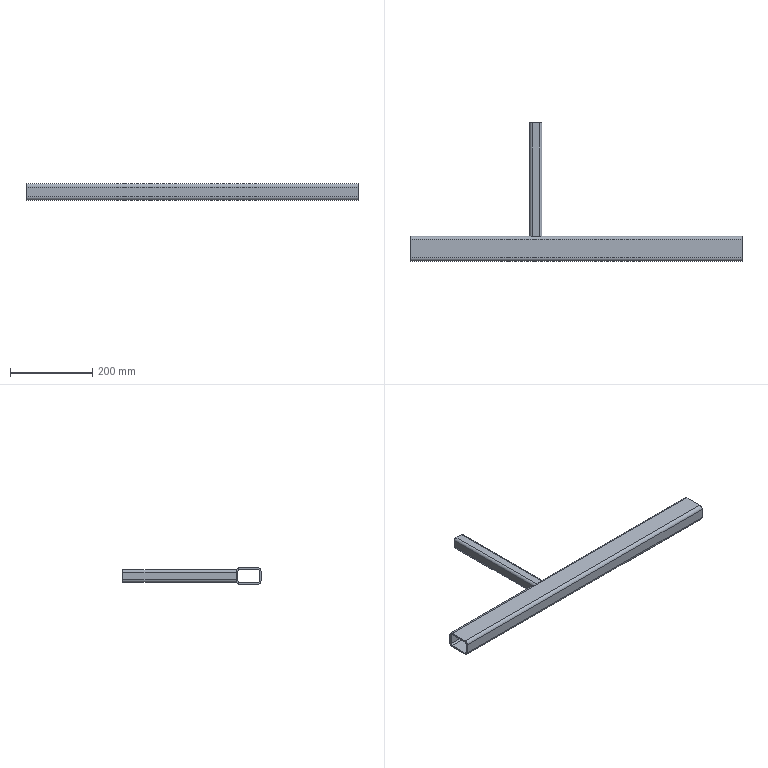Part | SolidWorks | features WeldMemberFeat 2, WeldCornerFeat 1, WeldmentFeature 1 | 2 solids | 36 faces | box 805 x 335 x 40 mm | volume 647000 mm3 | plane 20 | cylinder 16 | commonest cylinder face diameters 5.6 x4 8 x4 12 x4 16 x4
STEP:
#1=CARTESIAN_POINT('',(0.,-22.,20.));
#2=VERTEX_POINT('',#1);
#3=CARTESIAN_POINT('',(0.,-30.,12.));
#4=VERTEX_POINT('',#3);
#5=CARTESIAN_POINT('',(0.,-22.,12.));
#6=DIRECTION('',(1.,0.,0.));
#7=DIRECTION('',(0.,0.,-1.));
#8=AXIS2_PLACEMENT_3D('',#5,#6,#7);
#9=CIRCLE('',#8,8.);
#10=EDGE_CURVE('',#2,#4,#9,.T.);
#11=ORIENTED_EDGE('',*,*,#10,.T.);
#12=CARTESIAN_POINT('',(805.,-30.,12.));
#13=VERTEX_POINT('',#12);
#14=CARTESIAN_POINT('',(805.,-30.,12.));
#15=DIRECTION('',(-1.,0.,0.));
#16=VECTOR('',#15,1000.);
#17=LINE('',#14,#16);
#18=EDGE_CURVE('',#13,#4,#17,.T.);
#19=ORIENTED_EDGE('',*,*,#18,.F.);
#20=CARTESIAN_POINT('',(805.,-22.,20.));
#21=VERTEX_POINT('',#20);
#22=CARTESIAN_POINT('',(805.,-22.,12.));
#23=DIRECTION('',(1.,0.,0.));
#24=DIRECTION('',(0.,0.,-1.));
#25=AXIS2_PLACEMENT_3D('',#22,#23,#24);
#26=CIRCLE('',#25,8.);
#27=EDGE_CURVE('',#21,#13,#26,.T.);
#28=ORIENTED_EDGE('',*,*,#27,.F.);
#29=CARTESIAN_POINT('',(805.,-22.,20.));
#30=DIRECTION('',(-1.,0.,0.));
#31=VECTOR('',#30,1000.);
#32=LINE('',#29,#31);
#33=EDGE_CURVE('',#21,#2,#32,.T.);
#34=ORIENTED_EDGE('',*,*,#33,.T.);
#35=EDGE_LOOP('',(#11,#19,#28,#34));
#36=FACE_OUTER_BOUND('',#35,.T.);
#37=CARTESIAN_POINT('',(805.,-22.,12.));
#38=DIRECTION('',(-1.,0.,0.));
#39=DIRECTION('',(0.,0.,1.));
#40=AXIS2_PLACEMENT_3D('',#37,#38,#39);
#41=CYLINDRICAL_SURFACE('',#40,8.);
#42=ADVANCED_FACE('',(#36),#41,.T.);
#43=CARTESIAN_POINT('',(0.,-30.,-12.));
#44=VERTEX_POINT('',#43);
#45=CARTESIAN_POINT('',(0.,-30.,12.));
#46=DIRECTION('',(0.,0.,-1.));
#47=VECTOR('',#46,1000.);
#48=LINE('',#45,#47);
#49=EDGE_CURVE('',#4,#44,#48,.T.);
#50=ORIENTED_EDGE('',*,*,#49,.T.);
#51=CARTESIAN_POINT('',(805.,-30.,-12.));
#52=VERTEX_POINT('',#51);
#53=CARTESIAN_POINT('',(805.,-30.,-12.));
#54=DIRECTION('',(-1.,0.,0.));
#55=VECTOR('',#54,1000.);
#56=LINE('',#53,#55);
#57=EDGE_CURVE('',#52,#44,#56,.T.);
#58=ORIENTED_EDGE('',*,*,#57,.F.);
#59=CARTESIAN_POINT('',(805.,-30.,12.));
#60=DIRECTION('',(0.,0.,-1.));
#61=VECTOR('',#60,1000.);
#62=LINE('',#59,#61);
#63=EDGE_CURVE('',#13,#52,#62,.T.);
#64=ORIENTED_EDGE('',*,*,#63,.F.);
#65=ORIENTED_EDGE('',*,*,#18,.T.);
#66=EDGE_LOOP('',(#50,#58,#64,#65));
#67=FACE_OUTER_BOUND('',#66,.T.);
#68=CARTESIAN_POINT('',(805.,-30.,12.));
#69=DIRECTION('',(0.,1.,0.));
#70=DIRECTION('',(0.,0.,1.));
#71=AXIS2_PLACEMENT_3D('',#68,#69,#70);
#72=PLANE('',#71);
#73=ADVANCED_FACE('',(#67),#72,.F.);
#74=CARTESIAN_POINT('',(0.,-22.,-20.));
#75=VERTEX_POINT('',#74);
#76=CARTESIAN_POINT('',(0.,-22.,-12.));
#77=DIRECTION('',(1.,0.,0.));
#78=DIRECTION('',(0.,0.,-1.));
#79=AXIS2_PLACEMENT_3D('',#76,#77,#78);
#80=CIRCLE('',#79,8.);
#81=EDGE_CURVE('',#44,#75,#80,.T.);
#82=ORIENTED_EDGE('',*,*,#81,.T.);
#83=CARTESIAN_POINT('',(805.,-22.,-20.));
#84=VERTEX_POINT('',#83);
#85=CARTESIAN_POINT('',(805.,-22.,-20.));
#86=DIRECTION('',(-1.,0.,0.));
#87=VECTOR('',#86,1000.);
#88=LINE('',#85,#87);
#89=EDGE_CURVE('',#84,#75,#88,.T.);
#90=ORIENTED_EDGE('',*,*,#89,.F.);
#91=CARTESIAN_POINT('',(805.,-22.,-12.));
#92=DIRECTION('',(1.,0.,0.));
#93=DIRECTION('',(0.,0.,-1.));
#94=AXIS2_PLACEMENT_3D('',#91,#92,#93);
#95=CIRCLE('',#94,8.);
#96=EDGE_CURVE('',#52,#84,#95,.T.);
#97=ORIENTED_EDGE('',*,*,#96,.F.);
#98=ORIENTED_EDGE('',*,*,#57,.T.);
#99=EDGE_LOOP('',(#82,#90,#97,#98));
#100=FACE_OUTER_BOUND('',#99,.T.);
#101=CARTESIAN_POINT('',(805.,-22.,-12.));
#102=DIRECTION('',(-1.,0.,0.));
#103=DIRECTION('',(0.,0.,1.));
#104=AXIS2_PLACEMENT_3D('',#101,#102,#103);
#105=CYLINDRICAL_SURFACE('',#104,8.);
#106=ADVANCED_FACE('',(#100),#105,.T.);
#107=CARTESIAN_POINT('',(0.,22.,-20.));
#108=VERTEX_POINT('',#107);
#109=CARTESIAN_POINT('',(0.,22.,-20.));
#110=DIRECTION('',(0.,1.,0.));
#111=VECTOR('',#110,1000.);
#112=LINE('',#109,#111);
#113=EDGE_CURVE('',#75,#108,#112,.T.);
#114=ORIENTED_EDGE('',*,*,#113,.T.);
#115=CARTESIAN_POINT('',(805.,22.,-20.));
#116=VERTEX_POINT('',#115);
#117=CARTESIAN_POINT('',(805.,22.,-20.));
#118=DIRECTION('',(-1.,0.,0.));
#119=VECTOR('',#118,1000.);
#120=LINE('',#117,#119);
#121=EDGE_CURVE('',#116,#108,#120,.T.);
#122=ORIENTED_EDGE('',*,*,#121,.F.);
#123=CARTESIAN_POINT('',(805.,22.,-20.));
#124=DIRECTION('',(0.,1.,0.));
#125=VECTOR('',#124,1000.);
#126=LINE('',#123,#125);
#127=EDGE_CURVE('',#84,#116,#126,.T.);
#128=ORIENTED_EDGE('',*,*,#127,.F.);
#129=ORIENTED_EDGE('',*,*,#89,.T.);
#130=EDGE_LOOP('',(#114,#122,#128,#129));
#131=FACE_OUTER_BOUND('',#130,.T.);
#132=CARTESIAN_POINT('',(805.,22.,-20.));
#133=DIRECTION('',(0.,0.,1.));
#134=DIRECTION('',(0.,-1.,0.));
#135=AXIS2_PLACEMENT_3D('',#132,#133,#134);
#136=PLANE('',#135);
#137=ADVANCED_FACE('',(#131),#136,.F.);
#138=CARTESIAN_POINT('',(0.,30.,-12.));
#139=VERTEX_POINT('',#138);
#140=CARTESIAN_POINT('',(0.,22.,-12.));
#141=DIRECTION('',(1.,0.,0.));
#142=DIRECTION('',(0.,0.,-1.));
#143=AXIS2_PLACEMENT_3D('',#140,#141,#142);
#144=CIRCLE('',#143,8.);
#145=EDGE_CURVE('',#108,#139,#144,.T.);
#146=ORIENTED_EDGE('',*,*,#145,.T.);
#147=CARTESIAN_POINT('',(805.,30.,-12.));
#148=VERTEX_POINT('',#147);
#149=CARTESIAN_POINT('',(805.,30.,-12.));
#150=DIRECTION('',(-1.,0.,0.));
#151=VECTOR('',#150,1000.);
#152=LINE('',#149,#151);
#153=EDGE_CURVE('',#148,#139,#152,.T.);
#154=ORIENTED_EDGE('',*,*,#153,.F.);
#155=CARTESIAN_POINT('',(805.,22.,-12.));
#156=DIRECTION('',(1.,0.,0.));
#157=DIRECTION('',(0.,0.,-1.));
#158=AXIS2_PLACEMENT_3D('',#155,#156,#157);
#159=CIRCLE('',#158,8.);
#160=EDGE_CURVE('',#116,#148,#159,.T.);
#161=ORIENTED_EDGE('',*,*,#160,.F.);
#162=ORIENTED_EDGE('',*,*,#121,.T.);
#163=EDGE_LOOP('',(#146,#154,#161,#162));
#164=FACE_OUTER_BOUND('',#163,.T.);
#165=CARTESIAN_POINT('',(805.,22.,-12.));
#166=DIRECTION('',(-1.,0.,0.));
#167=DIRECTION('',(0.,0.,1.));
#168=AXIS2_PLACEMENT_3D('',#165,#166,#167);
#169=CYLINDRICAL_SURFACE('',#168,8.);
#170=ADVANCED_FACE('',(#164),#169,.T.);
#171=CARTESIAN_POINT('',(0.,30.,12.));
#172=VERTEX_POINT('',#171);
#173=CARTESIAN_POINT('',(0.,30.,-12.));
#174=DIRECTION('',(0.,0.,1.));
#175=VECTOR('',#174,1000.);
#176=LINE('',#173,#175);
#177=EDGE_CURVE('',#139,#172,#176,.T.);
#178=ORIENTED_EDGE('',*,*,#177,.T.);
#179=CARTESIAN_POINT('',(805.,30.,12.));
#180=VERTEX_POINT('',#179);
#181=CARTESIAN_POINT('',(805.,30.,12.));
#182=DIRECTION('',(-1.,0.,0.));
#183=VECTOR('',#182,1000.);
#184=LINE('',#181,#183);
#185=EDGE_CURVE('',#180,#172,#184,.T.);
#186=ORIENTED_EDGE('',*,*,#185,.F.);
#187=CARTESIAN_POINT('',(805.,30.,-12.));
#188=DIRECTION('',(0.,0.,1.));
#189=VECTOR('',#188,1000.);
#190=LINE('',#187,#189);
#191=EDGE_CURVE('',#148,#180,#190,.T.);
#192=ORIENTED_EDGE('',*,*,#191,.F.);
#193=ORIENTED_EDGE('',*,*,#153,.T.);
#194=EDGE_LOOP('',(#178,#186,#192,#193));
#195=FACE_OUTER_BOUND('',#194,.T.);
#196=CARTESIAN_POINT('',(805.,30.,-12.));
#197=DIRECTION('',(0.,-1.,0.));
#198=DIRECTION('',(0.,0.,-1.));
#199=AXIS2_PLACEMENT_3D('',#196,#197,#198);
#200=PLANE('',#199);
#201=ADVANCED_FACE('',(#195),#200,.F.);
#202=CARTESIAN_POINT('',(0.,22.,20.));
#203=VERTEX_POINT('',#202);
#204=CARTESIAN_POINT('',(0.,22.,12.));
#205=DIRECTION('',(1.,0.,0.));
#206=DIRECTION('',(0.,0.,-1.));
#207=AXIS2_PLACEMENT_3D('',#204,#205,#206);
#208=CIRCLE('',#207,8.);
#209=EDGE_CURVE('',#172,#203,#208,.T.);
#210=ORIENTED_EDGE('',*,*,#209,.T.);
#211=CARTESIAN_POINT('',(805.,22.,20.));
#212=VERTEX_POINT('',#211);
#213=CARTESIAN_POINT('',(805.,22.,20.));
#214=DIRECTION('',(-1.,0.,0.));
#215=VECTOR('',#214,1000.);
#216=LINE('',#213,#215);
#217=EDGE_CURVE('',#212,#203,#216,.T.);
#218=ORIENTED_EDGE('',*,*,#217,.F.);
#219=CARTESIAN_POINT('',(805.,22.,12.));
#220=DIRECTION('',(1.,0.,0.));
#221=DIRECTION('',(0.,0.,-1.));
#222=AXIS2_PLACEMENT_3D('',#219,#220,#221);
#223=CIRCLE('',#222,8.);
#224=EDGE_CURVE('',#180,#212,#223,.T.);
#225=ORIENTED_EDGE('',*,*,#224,.F.);
#226=ORIENTED_EDGE('',*,*,#185,.T.);
#227=EDGE_LOOP('',(#210,#218,#225,#226));
#228=FACE_OUTER_BOUND('',#227,.T.);
#229=CARTESIAN_POINT('',(805.,22.,12.));
#230=DIRECTION('',(-1.,0.,0.));
#231=DIRECTION('',(0.,0.,1.));
#232=AXIS2_PLACEMENT_3D('',#229,#230,#231);
#233=CYLINDRICAL_SURFACE('',#232,8.);
#234=ADVANCED_FACE('',(#228),#233,.T.);
#235=CARTESIAN_POINT('',(0.,-26.,-12.));
#236=VERTEX_POINT('',#235);
#237=CARTESIAN_POINT('',(0.,-22.,-16.));
#238=VERTEX_POINT('',#237);
#239=CARTESIAN_POINT('',(0.,-22.,-12.));
#240=DIRECTION('',(1.,0.,0.));
#241=DIRECTION('',(0.,0.,-1.));
#242=AXIS2_PLACEMENT_3D('',#239,#240,#241);
#243=CIRCLE('',#242,4.);
#244=EDGE_CURVE('',#236,#238,#243,.T.);
#245=ORIENTED_EDGE('',*,*,#244,.F.);
#246=CARTESIAN_POINT('',(805.,-26.,-12.));
#247=VERTEX_POINT('',#246);
#248=CARTESIAN_POINT('',(805.,-26.,-12.));
#249=DIRECTION('',(-1.,0.,0.));
#250=VECTOR('',#249,1000.);
#251=LINE('',#248,#250);
#252=EDGE_CURVE('',#247,#236,#251,.T.);
#253=ORIENTED_EDGE('',*,*,#252,.F.);
#254=CARTESIAN_POINT('',(805.,-22.,-16.));
#255=VERTEX_POINT('',#254);
#256=CARTESIAN_POINT('',(805.,-22.,-12.));
#257=DIRECTION('',(1.,0.,0.));
#258=DIRECTION('',(0.,0.,-1.));
#259=AXIS2_PLACEMENT_3D('',#256,#257,#258);
#260=CIRCLE('',#259,4.);
#261=EDGE_CURVE('',#247,#255,#260,.T.);
#262=ORIENTED_EDGE('',*,*,#261,.T.);
#263=CARTESIAN_POINT('',(805.,-22.,-16.));
#264=DIRECTION('',(-1.,0.,0.));
#265=VECTOR('',#264,1000.);
#266=LINE('',#263,#265);
#267=EDGE_CURVE('',#255,#238,#266,.T.);
#268=ORIENTED_EDGE('',*,*,#267,.T.);
#269=EDGE_LOOP('',(#245,#253,#262,#268));
#270=FACE_OUTER_BOUND('',#269,.T.);
#271=CARTESIAN_POINT('',(805.,-22.,-12.));
#272=DIRECTION('',(-1.,0.,0.));
#273=DIRECTION('',(0.,0.,1.));
#274=AXIS2_PLACEMENT_3D('',#271,#272,#273);
#275=CYLINDRICAL_SURFACE('',#274,4.);
#276=ADVANCED_FACE('',(#270),#275,.F.);
#277=CARTESIAN_POINT('',(0.,-26.,12.));
#278=VERTEX_POINT('',#277);
#279=CARTESIAN_POINT('',(0.,-26.,12.));
#280=DIRECTION('',(0.,0.,-1.));
#281=VECTOR('',#280,1000.);
#282=LINE('',#279,#281);
#283=EDGE_CURVE('',#278,#236,#282,.T.);
#284=ORIENTED_EDGE('',*,*,#283,.F.);
#285=CARTESIAN_POINT('',(805.,-26.,12.));
#286=VERTEX_POINT('',#285);
#287=CARTESIAN_POINT('',(805.,-26.,12.));
#288=DIRECTION('',(-1.,0.,0.));
#289=VECTOR('',#288,1000.);
#290=LINE('',#287,#289);
#291=EDGE_CURVE('',#286,#278,#290,.T.);
#292=ORIENTED_EDGE('',*,*,#291,.F.);
#293=CARTESIAN_POINT('',(805.,-26.,12.));
#294=DIRECTION('',(0.,0.,-1.));
#295=VECTOR('',#294,1000.);
#296=LINE('',#293,#295);
#297=EDGE_CURVE('',#286,#247,#296,.T.);
#298=ORIENTED_EDGE('',*,*,#297,.T.);
#299=ORIENTED_EDGE('',*,*,#252,.T.);
#300=EDGE_LOOP('',(#284,#292,#298,#299));
#301=FACE_OUTER_BOUND('',#300,.T.);
#302=CARTESIAN_POINT('',(805.,-26.,12.));
#303=DIRECTION('',(0.,1.,0.));
#304=DIRECTION('',(0.,0.,1.));
#305=AXIS2_PLACEMENT_3D('',#302,#303,#304);
#306=PLANE('',#305);
#307=ADVANCED_FACE('',(#301),#306,.T.);
#308=CARTESIAN_POINT('',(0.,-22.,16.));
#309=VERTEX_POINT('',#308);
#310=CARTESIAN_POINT('',(0.,-22.,12.));
#311=DIRECTION('',(1.,0.,0.));
#312=DIRECTION('',(0.,0.,-1.));
#313=AXIS2_PLACEMENT_3D('',#310,#311,#312);
#314=CIRCLE('',#313,4.);
#315=EDGE_CURVE('',#309,#278,#314,.T.);
#316=ORIENTED_EDGE('',*,*,#315,.F.);
#317=CARTESIAN_POINT('',(805.,-22.,16.));
#318=VERTEX_POINT('',#317);
#319=CARTESIAN_POINT('',(805.,-22.,16.));
#320=DIRECTION('',(-1.,0.,0.));
#321=VECTOR('',#320,1000.);
#322=LINE('',#319,#321);
#323=EDGE_CURVE('',#318,#309,#322,.T.);
#324=ORIENTED_EDGE('',*,*,#323,.F.);
#325=CARTESIAN_POINT('',(805.,-22.,12.));
#326=DIRECTION('',(1.,0.,0.));
#327=DIRECTION('',(0.,0.,-1.));
#328=AXIS2_PLACEMENT_3D('',#325,#326,#327);
#329=CIRCLE('',#328,4.);
#330=EDGE_CURVE('',#318,#286,#329,.T.);
#331=ORIENTED_EDGE('',*,*,#330,.T.);
#332=ORIENTED_EDGE('',*,*,#291,.T.);
#333=EDGE_LOOP('',(#316,#324,#331,#332));
#334=FACE_OUTER_BOUND('',#333,.T.);
#335=CARTESIAN_POINT('',(805.,-22.,12.));
#336=DIRECTION('',(-1.,0.,0.));
#337=DIRECTION('',(0.,0.,1.));
#338=AXIS2_PLACEMENT_3D('',#335,#336,#337);
#339=CYLINDRICAL_SURFACE('',#338,4.);
#340=ADVANCED_FACE('',(#334),#339,.F.);
#341=CARTESIAN_POINT('',(0.,22.,16.));
#342=VERTEX_POINT('',#341);
#343=CARTESIAN_POINT('',(0.,-22.,16.));
#344=DIRECTION('',(0.,-1.,0.));
#345=VECTOR('',#344,1000.);
#346=LINE('',#343,#345);
#347=EDGE_CURVE('',#342,#309,#346,.T.);
#348=ORIENTED_EDGE('',*,*,#347,.F.);
#349=CARTESIAN_POINT('',(805.,22.,16.));
#350=VERTEX_POINT('',#349);
#351=CARTESIAN_POINT('',(805.,22.,16.));
#352=DIRECTION('',(-1.,0.,0.));
#353=VECTOR('',#352,1000.);
#354=LINE('',#351,#353);
#355=EDGE_CURVE('',#350,#342,#354,.T.);
#356=ORIENTED_EDGE('',*,*,#355,.F.);
#357=CARTESIAN_POINT('',(805.,-22.,16.));
#358=DIRECTION('',(0.,-1.,0.));
#359=VECTOR('',#358,1000.);
#360=LINE('',#357,#359);
#361=EDGE_CURVE('',#350,#318,#360,.T.);
#362=ORIENTED_EDGE('',*,*,#361,.T.);
#363=ORIENTED_EDGE('',*,*,#323,.T.);
#364=EDGE_LOOP('',(#348,#356,#362,#363));
#365=FACE_OUTER_BOUND('',#364,.T.);
#366=CARTESIAN_POINT('',(805.,-22.,16.));
#367=DIRECTION('',(0.,0.,-1.));
#368=DIRECTION('',(0.,1.,0.));
#369=AXIS2_PLACEMENT_3D('',#366,#367,#368);
#370=PLANE('',#369);
#371=ADVANCED_FACE('',(#365),#370,.T.);
#372=CARTESIAN_POINT('',(0.,26.,12.));
#373=VERTEX_POINT('',#372);
#374=CARTESIAN_POINT('',(0.,22.,12.));
#375=DIRECTION('',(1.,0.,0.));
#376=DIRECTION('',(0.,0.,-1.));
#377=AXIS2_PLACEMENT_3D('',#374,#375,#376);
#378=CIRCLE('',#377,4.);
#379=EDGE_CURVE('',#373,#342,#378,.T.);
#380=ORIENTED_EDGE('',*,*,#379,.F.);
#381=CARTESIAN_POINT('',(805.,26.,12.));
#382=VERTEX_POINT('',#381);
#383=CARTESIAN_POINT('',(805.,26.,12.));
#384=DIRECTION('',(-1.,0.,0.));
#385=VECTOR('',#384,1000.);
#386=LINE('',#383,#385);
#387=EDGE_CURVE('',#382,#373,#386,.T.);
#388=ORIENTED_EDGE('',*,*,#387,.F.);
#389=CARTESIAN_POINT('',(805.,22.,12.));
#390=DIRECTION('',(1.,0.,0.));
#391=DIRECTION('',(0.,0.,-1.));
#392=AXIS2_PLACEMENT_3D('',#389,#390,#391);
#393=CIRCLE('',#392,4.);
#394=EDGE_CURVE('',#382,#350,#393,.T.);
#395=ORIENTED_EDGE('',*,*,#394,.T.);
#396=ORIENTED_EDGE('',*,*,#355,.T.);
#397=EDGE_LOOP('',(#380,#388,#395,#396));
#398=FACE_OUTER_BOUND('',#397,.T.);
#399=CARTESIAN_POINT('',(805.,22.,12.));
#400=DIRECTION('',(-1.,0.,0.));
#401=DIRECTION('',(0.,0.,1.));
#402=AXIS2_PLACEMENT_3D('',#399,#400,#401);
#403=CYLINDRICAL_SURFACE('',#402,4.);
#404=ADVANCED_FACE('',(#398),#403,.F.);
#405=CARTESIAN_POINT('',(0.,26.,-12.));
#406=VERTEX_POINT('',#405);
#407=CARTESIAN_POINT('',(0.,26.,-12.));
#408=DIRECTION('',(0.,0.,1.));
#409=VECTOR('',#408,1000.);
#410=LINE('',#407,#409);
#411=EDGE_CURVE('',#406,#373,#410,.T.);
#412=ORIENTED_EDGE('',*,*,#411,.F.);
#413=CARTESIAN_POINT('',(805.,26.,-12.));
#414=VERTEX_POINT('',#413);
#415=CARTESIAN_POINT('',(805.,26.,-12.));
#416=DIRECTION('',(-1.,0.,0.));
#417=VECTOR('',#416,1000.);
#418=LINE('',#415,#417);
#419=EDGE_CURVE('',#414,#406,#418,.T.);
#420=ORIENTED_EDGE('',*,*,#419,.F.);
#421=CARTESIAN_POINT('',(805.,26.,-12.));
#422=DIRECTION('',(0.,0.,1.));
#423=VECTOR('',#422,1000.);
#424=LINE('',#421,#423);
#425=EDGE_CURVE('',#414,#382,#424,.T.);
#426=ORIENTED_EDGE('',*,*,#425,.T.);
#427=ORIENTED_EDGE('',*,*,#387,.T.);
#428=EDGE_LOOP('',(#412,#420,#426,#427));
#429=FACE_OUTER_BOUND('',#428,.T.);
#430=CARTESIAN_POINT('',(805.,26.,-12.));
#431=DIRECTION('',(0.,-1.,0.));
#432=DIRECTION('',(0.,0.,-1.));
#433=AXIS2_PLACEMENT_3D('',#430,#431,#432);
#434=PLANE('',#433);
#435=ADVANCED_FACE('',(#429),#434,.T.);
#436=CARTESIAN_POINT('',(0.,22.,-16.));
#437=VERTEX_POINT('',#436);
#438=CARTESIAN_POINT('',(0.,22.,-12.));
#439=DIRECTION('',(1.,0.,0.));
#440=DIRECTION('',(0.,0.,-1.));
#441=AXIS2_PLACEMENT_3D('',#438,#439,#440);
#442=CIRCLE('',#441,4.);
#443=EDGE_CURVE('',#437,#406,#442,.T.);
#444=ORIENTED_EDGE('',*,*,#443,.F.);
#445=CARTESIAN_POINT('',(805.,22.,-16.));
#446=VERTEX_POINT('',#445);
#447=CARTESIAN_POINT('',(805.,22.,-16.));
#448=DIRECTION('',(-1.,0.,0.));
#449=VECTOR('',#448,1000.);
#450=LINE('',#447,#449);
#451=EDGE_CURVE('',#446,#437,#450,.T.);
#452=ORIENTED_EDGE('',*,*,#451,.F.);
#453=CARTESIAN_POINT('',(805.,22.,-12.));
#454=DIRECTION('',(1.,0.,0.));
#455=DIRECTION('',(0.,0.,-1.));
#456=AXIS2_PLACEMENT_3D('',#453,#454,#455);
#457=CIRCLE('',#456,4.);
#458=EDGE_CURVE('',#446,#414,#457,.T.);
#459=ORIENTED_EDGE('',*,*,#458,.T.);
#460=ORIENTED_EDGE('',*,*,#419,.T.);
#461=EDGE_LOOP('',(#444,#452,#459,#460));
#462=FACE_OUTER_BOUND('',#461,.T.);
#463=CARTESIAN_POINT('',(805.,22.,-12.));
#464=DIRECTION('',(-1.,0.,0.));
#465=DIRECTION('',(0.,0.,1.));
#466=AXIS2_PLACEMENT_3D('',#463,#464,#465);
#467=CYLINDRICAL_SURFACE('',#466,4.);
#468=ADVANCED_FACE('',(#462),#467,.F.);
#469=CARTESIAN_POINT('',(0.,22.,-16.));
#470=DIRECTION('',(0.,1.,0.));
#471=VECTOR('',#470,1000.);
#472=LINE('',#469,#471);
#473=EDGE_CURVE('',#238,#437,#472,.T.);
#474=ORIENTED_EDGE('',*,*,#473,.F.);
#475=ORIENTED_EDGE('',*,*,#267,.F.);
#476=CARTESIAN_POINT('',(805.,22.,-16.));
#477=DIRECTION('',(0.,1.,0.));
#478=VECTOR('',#477,1000.);
#479=LINE('',#476,#478);
#480=EDGE_CURVE('',#255,#446,#479,.T.);
#481=ORIENTED_EDGE('',*,*,#480,.T.);
#482=ORIENTED_EDGE('',*,*,#451,.T.);
#483=EDGE_LOOP('',(#474,#475,#481,#482));
#484=FACE_OUTER_BOUND('',#483,.T.);
#485=CARTESIAN_POINT('',(805.,22.,-16.));
#486=DIRECTION('',(0.,0.,1.));
#487=DIRECTION('',(0.,-1.,0.));
#488=AXIS2_PLACEMENT_3D('',#485,#486,#487);
#489=PLANE('',#488);
#490=ADVANCED_FACE('',(#484),#489,.T.);
#491=CARTESIAN_POINT('',(0.,-22.,20.));
#492=DIRECTION('',(0.,-1.,0.));
#493=VECTOR('',#492,1000.);
#494=LINE('',#491,#493);
#495=EDGE_CURVE('',#203,#2,#494,.T.);
#496=ORIENTED_EDGE('',*,*,#495,.T.);
#497=ORIENTED_EDGE('',*,*,#33,.F.);
#498=CARTESIAN_POINT('',(805.,-22.,20.));
#499=DIRECTION('',(0.,-1.,0.));
#500=VECTOR('',#499,1000.);
#501=LINE('',#498,#500);
#502=EDGE_CURVE('',#212,#21,#501,.T.);
#503=ORIENTED_EDGE('',*,*,#502,.F.);
#504=ORIENTED_EDGE('',*,*,#217,.T.);
#505=EDGE_LOOP('',(#496,#497,#503,#504));
#506=FACE_OUTER_BOUND('',#505,.T.);
#507=CARTESIAN_POINT('',(805.,-22.,20.));
#508=DIRECTION('',(0.,0.,-1.));
#509=DIRECTION('',(0.,1.,0.));
#510=AXIS2_PLACEMENT_3D('',#507,#508,#509);
#511=PLANE('',#510);
#512=ADVANCED_FACE('',(#506),#511,.F.);
#513=ORIENTED_EDGE('',*,*,#261,.F.);
#514=ORIENTED_EDGE('',*,*,#297,.F.);
#515=ORIENTED_EDGE('',*,*,#330,.F.);
#516=ORIENTED_EDGE('',*,*,#361,.F.);
#517=ORIENTED_EDGE('',*,*,#394,.F.);
#518=ORIENTED_EDGE('',*,*,#425,.F.);
#519=ORIENTED_EDGE('',*,*,#458,.F.);
#520=ORIENTED_EDGE('',*,*,#480,.F.);
#521=EDGE_LOOP('',(#513,#514,#515,#516,#517,#518,#519,#520));
#522=FACE_BOUND('',#521,.T.);
#523=ORIENTED_EDGE('',*,*,#27,.T.);
#524=ORIENTED_EDGE('',*,*,#63,.T.);
#525=ORIENTED_EDGE('',*,*,#96,.T.);
#526=ORIENTED_EDGE('',*,*,#127,.T.);
#527=ORIENTED_EDGE('',*,*,#160,.T.);
#528=ORIENTED_EDGE('',*,*,#191,.T.);
#529=ORIENTED_EDGE('',*,*,#224,.T.);
#530=ORIENTED_EDGE('',*,*,#502,.T.);
#531=EDGE_LOOP('',(#523,#524,#525,#526,#527,#528,#529,#530));
#532=FACE_OUTER_BOUND('',#531,.T.);
#533=CARTESIAN_POINT('',(805.,-22.,12.));
#534=DIRECTION('',(1.,0.,0.));
#535=DIRECTION('',(0.,0.,-1.));
#536=AXIS2_PLACEMENT_3D('',#533,#534,#535);
#537=PLANE('',#536);
#538=ADVANCED_FACE('',(#522,#532),#537,.T.);
#539=ORIENTED_EDGE('',*,*,#244,.T.);
#540=ORIENTED_EDGE('',*,*,#473,.T.);
#541=ORIENTED_EDGE('',*,*,#443,.T.);
#542=ORIENTED_EDGE('',*,*,#411,.T.);
#543=ORIENTED_EDGE('',*,*,#379,.T.);
#544=ORIENTED_EDGE('',*,*,#347,.T.);
#545=ORIENTED_EDGE('',*,*,#315,.T.);
#546=ORIENTED_EDGE('',*,*,#283,.T.);
#547=EDGE_LOOP('',(#539,#540,#541,#542,#543,#544,#545,#546));
#548=FACE_BOUND('',#547,.T.);
#549=ORIENTED_EDGE('',*,*,#10,.F.);
#550=ORIENTED_EDGE('',*,*,#495,.F.);
#551=ORIENTED_EDGE('',*,*,#209,.F.);
#552=ORIENTED_EDGE('',*,*,#177,.F.);
#553=ORIENTED_EDGE('',*,*,#145,.F.);
#554=ORIENTED_EDGE('',*,*,#113,.F.);
#555=ORIENTED_EDGE('',*,*,#81,.F.);
#556=ORIENTED_EDGE('',*,*,#49,.F.);
#557=EDGE_LOOP('',(#549,#550,#551,#552,#553,#554,#555,#556));
#558=FACE_OUTER_BOUND('',#557,.T.);
#559=CARTESIAN_POINT('',(0.,-22.,12.));
#560=DIRECTION('',(1.,0.,0.));
#561=DIRECTION('',(0.,0.,-1.));
#562=AXIS2_PLACEMENT_3D('',#559,#560,#561);
#563=PLANE('',#562);
#564=ADVANCED_FACE('',(#548,#558),#563,.F.);
#565=CLOSED_SHELL('',(#42,#73,#106,#137,#170,#201,#234,#276,#307,#340,#371,#404,#435,#468,#490,#512,#538,#564));
#566=MANIFOLD_SOLID_BREP('',#565);
#567=CARTESIAN_POINT('',(290.,305.,9.));
#568=VERTEX_POINT('',#567);
#569=CARTESIAN_POINT('',(296.,305.,15.));
#570=VERTEX_POINT('',#569);
#571=CARTESIAN_POINT('',(296.,305.,9.));
#572=DIRECTION('',(0.,1.,0.));
#573=DIRECTION('',(0.,0.,1.));
#574=AXIS2_PLACEMENT_3D('',#571,#572,#573);
#575=CIRCLE('',#574,6.);
#576=EDGE_CURVE('',#568,#570,#575,.T.);
#577=ORIENTED_EDGE('',*,*,#576,.F.);
#578=CARTESIAN_POINT('',(290.,30.,9.));
#579=VERTEX_POINT('',#578);
#580=CARTESIAN_POINT('',(290.,305.,9.));
#581=DIRECTION('',(0.,-1.,0.));
#582=VECTOR('',#581,1000.);
#583=LINE('',#580,#582);
#584=EDGE_CURVE('',#568,#579,#583,.T.);
#585=ORIENTED_EDGE('',*,*,#584,.T.);
#586=CARTESIAN_POINT('',(296.,30.,15.));
#587=VERTEX_POINT('',#586);
#588=CARTESIAN_POINT('',(296.,30.,9.));
#589=DIRECTION('',(0.,-1.,0.));
#590=DIRECTION('',(0.,0.,-1.));
#591=AXIS2_PLACEMENT_3D('',#588,#589,#590);
#592=CIRCLE('',#591,6.);
#593=EDGE_CURVE('',#587,#579,#592,.T.);
#594=ORIENTED_EDGE('',*,*,#593,.F.);
#595=CARTESIAN_POINT('',(296.,305.,15.));
#596=DIRECTION('',(0.,-1.,0.));
#597=VECTOR('',#596,1000.);
#598=LINE('',#595,#597);
#599=EDGE_CURVE('',#570,#587,#598,.T.);
#600=ORIENTED_EDGE('',*,*,#599,.F.);
#601=EDGE_LOOP('',(#577,#585,#594,#600));
#602=FACE_OUTER_BOUND('',#601,.T.);
#603=CARTESIAN_POINT('',(296.,305.,9.));
#604=DIRECTION('',(0.,-1.,0.));
#605=DIRECTION('',(0.,0.,-1.));
#606=AXIS2_PLACEMENT_3D('',#603,#604,#605);
#607=CYLINDRICAL_SURFACE('',#606,6.);
#608=ADVANCED_FACE('',(#602),#607,.T.);
#609=CARTESIAN_POINT('',(314.,305.,15.));
#610=VERTEX_POINT('',#609);
#611=CARTESIAN_POINT('',(296.,305.,15.));
#612=DIRECTION('',(1.,0.,0.));
#613=VECTOR('',#612,1000.);
#614=LINE('',#611,#613);
#615=EDGE_CURVE('',#570,#610,#614,.T.);
#616=ORIENTED_EDGE('',*,*,#615,.F.);
#617=ORIENTED_EDGE('',*,*,#599,.T.);
#618=CARTESIAN_POINT('',(314.,30.,15.));
#619=VERTEX_POINT('',#618);
#620=CARTESIAN_POINT('',(296.,30.,15.));
#621=DIRECTION('',(-1.,0.,0.));
#622=VECTOR('',#621,1000.);
#623=LINE('',#620,#622);
#624=EDGE_CURVE('',#619,#587,#623,.T.);
#625=ORIENTED_EDGE('',*,*,#624,.F.);
#626=CARTESIAN_POINT('',(314.,305.,15.));
#627=DIRECTION('',(0.,-1.,0.));
#628=VECTOR('',#627,1000.);
#629=LINE('',#626,#628);
#630=EDGE_CURVE('',#610,#619,#629,.T.);
#631=ORIENTED_EDGE('',*,*,#630,.F.);
#632=EDGE_LOOP('',(#616,#617,#625,#631));
#633=FACE_OUTER_BOUND('',#632,.T.);
#634=CARTESIAN_POINT('',(296.,305.,15.));
#635=DIRECTION('',(0.,0.,-1.));
#636=DIRECTION('',(-1.,0.,0.));
#637=AXIS2_PLACEMENT_3D('',#634,#635,#636);
#638=PLANE('',#637);
#639=ADVANCED_FACE('',(#633),#638,.F.);
#640=CARTESIAN_POINT('',(320.,305.,9.));
#641=VERTEX_POINT('',#640);
#642=CARTESIAN_POINT('',(314.,305.,9.));
#643=DIRECTION('',(0.,1.,0.));
#644=DIRECTION('',(0.,0.,1.));
#645=AXIS2_PLACEMENT_3D('',#642,#643,#644);
#646=CIRCLE('',#645,6.);
#647=EDGE_CURVE('',#610,#641,#646,.T.);
#648=ORIENTED_EDGE('',*,*,#647,.F.);
#649=ORIENTED_EDGE('',*,*,#630,.T.);
#650=CARTESIAN_POINT('',(320.,30.,9.));
#651=VERTEX_POINT('',#650);
#652=CARTESIAN_POINT('',(314.,30.,9.));
#653=DIRECTION('',(0.,-1.,0.));
#654=DIRECTION('',(0.,0.,-1.));
#655=AXIS2_PLACEMENT_3D('',#652,#653,#654);
#656=CIRCLE('',#655,6.);
#657=EDGE_CURVE('',#651,#619,#656,.T.);
#658=ORIENTED_EDGE('',*,*,#657,.F.);
#659=CARTESIAN_POINT('',(320.,305.,9.));
#660=DIRECTION('',(0.,-1.,0.));
#661=VECTOR('',#660,1000.);
#662=LINE('',#659,#661);
#663=EDGE_CURVE('',#641,#651,#662,.T.);
#664=ORIENTED_EDGE('',*,*,#663,.F.);
#665=EDGE_LOOP('',(#648,#649,#658,#664));
#666=FACE_OUTER_BOUND('',#665,.T.);
#667=CARTESIAN_POINT('',(314.,305.,9.));
#668=DIRECTION('',(0.,-1.,0.));
#669=DIRECTION('',(0.,0.,-1.));
#670=AXIS2_PLACEMENT_3D('',#667,#668,#669);
#671=CYLINDRICAL_SURFACE('',#670,6.);
#672=ADVANCED_FACE('',(#666),#671,.T.);
#673=CARTESIAN_POINT('',(320.,305.,-9.));
#674=VERTEX_POINT('',#673);
#675=CARTESIAN_POINT('',(320.,305.,-9.));
#676=DIRECTION('',(0.,0.,-1.));
#677=VECTOR('',#676,1000.);
#678=LINE('',#675,#677);
#679=EDGE_CURVE('',#641,#674,#678,.T.);
#680=ORIENTED_EDGE('',*,*,#679,.F.);
#681=ORIENTED_EDGE('',*,*,#663,.T.);
#682=CARTESIAN_POINT('',(320.,30.,-9.));
#683=VERTEX_POINT('',#682);
#684=CARTESIAN_POINT('',(320.,30.,-9.));
#685=DIRECTION('',(0.,0.,1.));
#686=VECTOR('',#685,1000.);
#687=LINE('',#684,#686);
#688=EDGE_CURVE('',#683,#651,#687,.T.);
#689=ORIENTED_EDGE('',*,*,#688,.F.);
#690=CARTESIAN_POINT('',(320.,305.,-9.));
#691=DIRECTION('',(0.,-1.,0.));
#692=VECTOR('',#691,1000.);
#693=LINE('',#690,#692);
#694=EDGE_CURVE('',#674,#683,#693,.T.);
#695=ORIENTED_EDGE('',*,*,#694,.F.);
#696=EDGE_LOOP('',(#680,#681,#689,#695));
#697=FACE_OUTER_BOUND('',#696,.T.);
#698=CARTESIAN_POINT('',(320.,305.,-9.));
#699=DIRECTION('',(-1.,0.,0.));
#700=DIRECTION('',(0.,0.,1.));
#701=AXIS2_PLACEMENT_3D('',#698,#699,#700);
#702=PLANE('',#701);
#703=ADVANCED_FACE('',(#697),#702,.F.);
#704=CARTESIAN_POINT('',(314.,305.,-15.));
#705=VERTEX_POINT('',#704);
#706=CARTESIAN_POINT('',(314.,305.,-9.));
#707=DIRECTION('',(0.,1.,0.));
#708=DIRECTION('',(0.,0.,1.));
#709=AXIS2_PLACEMENT_3D('',#706,#707,#708);
#710=CIRCLE('',#709,6.);
#711=EDGE_CURVE('',#674,#705,#710,.T.);
#712=ORIENTED_EDGE('',*,*,#711,.F.);
#713=ORIENTED_EDGE('',*,*,#694,.T.);
#714=CARTESIAN_POINT('',(314.,30.,-15.));
#715=VERTEX_POINT('',#714);
#716=CARTESIAN_POINT('',(314.,30.,-9.));
#717=DIRECTION('',(0.,-1.,0.));
#718=DIRECTION('',(0.,0.,-1.));
#719=AXIS2_PLACEMENT_3D('',#716,#717,#718);
#720=CIRCLE('',#719,6.);
#721=EDGE_CURVE('',#715,#683,#720,.T.);
#722=ORIENTED_EDGE('',*,*,#721,.F.);
#723=CARTESIAN_POINT('',(314.,305.,-15.));
#724=DIRECTION('',(0.,-1.,0.));
#725=VECTOR('',#724,1000.);
#726=LINE('',#723,#725);
#727=EDGE_CURVE('',#705,#715,#726,.T.);
#728=ORIENTED_EDGE('',*,*,#727,.F.);
#729=EDGE_LOOP('',(#712,#713,#722,#728));
#730=FACE_OUTER_BOUND('',#729,.T.);
#731=CARTESIAN_POINT('',(314.,305.,-9.));
#732=DIRECTION('',(0.,-1.,0.));
#733=DIRECTION('',(0.,0.,-1.));
#734=AXIS2_PLACEMENT_3D('',#731,#732,#733);
#735=CYLINDRICAL_SURFACE('',#734,6.);
#736=ADVANCED_FACE('',(#730),#735,.T.);
#737=CARTESIAN_POINT('',(296.,305.,-15.));
#738=VERTEX_POINT('',#737);
#739=CARTESIAN_POINT('',(314.,305.,-15.));
#740=DIRECTION('',(-1.,0.,0.));
#741=VECTOR('',#740,1000.);
#742=LINE('',#739,#741);
#743=EDGE_CURVE('',#705,#738,#742,.T.);
#744=ORIENTED_EDGE('',*,*,#743,.F.);
#745=ORIENTED_EDGE('',*,*,#727,.T.);
#746=CARTESIAN_POINT('',(296.,30.,-15.));
#747=VERTEX_POINT('',#746);
#748=CARTESIAN_POINT('',(314.,30.,-15.));
#749=DIRECTION('',(1.,0.,0.));
#750=VECTOR('',#749,1000.);
#751=LINE('',#748,#750);
#752=EDGE_CURVE('',#747,#715,#751,.T.);
#753=ORIENTED_EDGE('',*,*,#752,.F.);
#754=CARTESIAN_POINT('',(296.,305.,-15.));
#755=DIRECTION('',(0.,-1.,0.));
#756=VECTOR('',#755,1000.);
#757=LINE('',#754,#756);
#758=EDGE_CURVE('',#738,#747,#757,.T.);
#759=ORIENTED_EDGE('',*,*,#758,.F.);
#760=EDGE_LOOP('',(#744,#745,#753,#759));
#761=FACE_OUTER_BOUND('',#760,.T.);
#762=CARTESIAN_POINT('',(314.,305.,-15.));
#763=DIRECTION('',(0.,0.,1.));
#764=DIRECTION('',(1.,0.,0.));
#765=AXIS2_PLACEMENT_3D('',#762,#763,#764);
#766=PLANE('',#765);
#767=ADVANCED_FACE('',(#761),#766,.F.);
#768=CARTESIAN_POINT('',(290.,305.,-9.));
#769=VERTEX_POINT('',#768);
#770=CARTESIAN_POINT('',(296.,305.,-9.));
#771=DIRECTION('',(0.,1.,0.));
#772=DIRECTION('',(0.,0.,1.));
#773=AXIS2_PLACEMENT_3D('',#770,#771,#772);
#774=CIRCLE('',#773,6.);
#775=EDGE_CURVE('',#738,#769,#774,.T.);
#776=ORIENTED_EDGE('',*,*,#775,.F.);
#777=ORIENTED_EDGE('',*,*,#758,.T.);
#778=CARTESIAN_POINT('',(290.,30.,-9.));
#779=VERTEX_POINT('',#778);
#780=CARTESIAN_POINT('',(296.,30.,-9.));
#781=DIRECTION('',(0.,-1.,0.));
#782=DIRECTION('',(0.,0.,-1.));
#783=AXIS2_PLACEMENT_3D('',#780,#781,#782);
#784=CIRCLE('',#783,6.);
#785=EDGE_CURVE('',#779,#747,#784,.T.);
#786=ORIENTED_EDGE('',*,*,#785,.F.);
#787=CARTESIAN_POINT('',(290.,305.,-9.));
#788=DIRECTION('',(0.,-1.,0.));
#789=VECTOR('',#788,1000.);
#790=LINE('',#787,#789);
#791=EDGE_CURVE('',#769,#779,#790,.T.);
#792=ORIENTED_EDGE('',*,*,#791,.F.);
#793=EDGE_LOOP('',(#776,#777,#786,#792));
#794=FACE_OUTER_BOUND('',#793,.T.);
#795=CARTESIAN_POINT('',(296.,305.,-9.));
#796=DIRECTION('',(0.,-1.,0.));
#797=DIRECTION('',(0.,0.,-1.));
#798=AXIS2_PLACEMENT_3D('',#795,#796,#797);
#799=CYLINDRICAL_SURFACE('',#798,6.);
#800=ADVANCED_FACE('',(#794),#799,.T.);
#801=CARTESIAN_POINT('',(314.,305.,11.8));
#802=VERTEX_POINT('',#801);
#803=CARTESIAN_POINT('',(314.,30.,11.8));
#804=VERTEX_POINT('',#803);
#805=CARTESIAN_POINT('',(314.,305.,11.8));
#806=DIRECTION('',(0.,-1.,0.));
#807=VECTOR('',#806,1000.);
#808=LINE('',#805,#807);
#809=EDGE_CURVE('',#802,#804,#808,.T.);
#810=ORIENTED_EDGE('',*,*,#809,.F.);
#811=CARTESIAN_POINT('',(316.8,305.,9.));
#812=VERTEX_POINT('',#811);
#813=CARTESIAN_POINT('',(314.,305.,9.));
#814=DIRECTION('',(0.,1.,0.));
#815=DIRECTION('',(0.,0.,1.));
#816=AXIS2_PLACEMENT_3D('',#813,#814,#815);
#817=CIRCLE('',#816,2.8);
#818=EDGE_CURVE('',#802,#812,#817,.T.);
#819=ORIENTED_EDGE('',*,*,#818,.T.);
#820=CARTESIAN_POINT('',(316.8,30.,9.));
#821=VERTEX_POINT('',#820);
#822=CARTESIAN_POINT('',(316.8,305.,9.));
#823=DIRECTION('',(0.,-1.,0.));
#824=VECTOR('',#823,1000.);
#825=LINE('',#822,#824);
#826=EDGE_CURVE('',#812,#821,#825,.T.);
#827=ORIENTED_EDGE('',*,*,#826,.T.);
#828=CARTESIAN_POINT('',(314.,30.,9.));
#829=DIRECTION('',(0.,-1.,0.));
#830=DIRECTION('',(0.,0.,-1.));
#831=AXIS2_PLACEMENT_3D('',#828,#829,#830);
#832=CIRCLE('',#831,2.8);
#833=EDGE_CURVE('',#821,#804,#832,.T.);
#834=ORIENTED_EDGE('',*,*,#833,.T.);
#835=EDGE_LOOP('',(#810,#819,#827,#834));
#836=FACE_OUTER_BOUND('',#835,.T.);
#837=CARTESIAN_POINT('',(314.,305.,9.));
#838=DIRECTION('',(0.,-1.,0.));
#839=DIRECTION('',(0.,0.,-1.));
#840=AXIS2_PLACEMENT_3D('',#837,#838,#839);
#841=CYLINDRICAL_SURFACE('',#840,2.8);
#842=ADVANCED_FACE('',(#836),#841,.F.);
#843=CARTESIAN_POINT('',(296.,305.,11.8));
#844=VERTEX_POINT('',#843);
#845=CARTESIAN_POINT('',(296.,30.,11.8));
#846=VERTEX_POINT('',#845);
#847=CARTESIAN_POINT('',(296.,305.,11.8));
#848=DIRECTION('',(0.,-1.,0.));
#849=VECTOR('',#848,1000.);
#850=LINE('',#847,#849);
#851=EDGE_CURVE('',#844,#846,#850,.T.);
#852=ORIENTED_EDGE('',*,*,#851,.F.);
#853=CARTESIAN_POINT('',(296.,305.,11.8));
#854=DIRECTION('',(1.,0.,0.));
#855=VECTOR('',#854,1000.);
#856=LINE('',#853,#855);
#857=EDGE_CURVE('',#844,#802,#856,.T.);
#858=ORIENTED_EDGE('',*,*,#857,.T.);
#859=ORIENTED_EDGE('',*,*,#809,.T.);
#860=CARTESIAN_POINT('',(296.,30.,11.8));
#861=DIRECTION('',(-1.,0.,0.));
#862=VECTOR('',#861,1000.);
#863=LINE('',#860,#862);
#864=EDGE_CURVE('',#804,#846,#863,.T.);
#865=ORIENTED_EDGE('',*,*,#864,.T.);
#866=EDGE_LOOP('',(#852,#858,#859,#865));
#867=FACE_OUTER_BOUND('',#866,.T.);
#868=CARTESIAN_POINT('',(296.,305.,11.8));
#869=DIRECTION('',(0.,0.,-1.));
#870=DIRECTION('',(-1.,0.,0.));
#871=AXIS2_PLACEMENT_3D('',#868,#869,#870);
#872=PLANE('',#871);
#873=ADVANCED_FACE('',(#867),#872,.T.);
#874=CARTESIAN_POINT('',(293.2,305.,9.));
#875=VERTEX_POINT('',#874);
#876=CARTESIAN_POINT('',(293.2,30.,9.));
#877=VERTEX_POINT('',#876);
#878=CARTESIAN_POINT('',(293.2,305.,9.));
#879=DIRECTION('',(0.,-1.,0.));
#880=VECTOR('',#879,1000.);
#881=LINE('',#878,#880);
#882=EDGE_CURVE('',#875,#877,#881,.T.);
#883=ORIENTED_EDGE('',*,*,#882,.F.);
#884=CARTESIAN_POINT('',(296.,305.,9.));
#885=DIRECTION('',(0.,1.,0.));
#886=DIRECTION('',(0.,0.,1.));
#887=AXIS2_PLACEMENT_3D('',#884,#885,#886);
#888=CIRCLE('',#887,2.8);
#889=EDGE_CURVE('',#875,#844,#888,.T.);
#890=ORIENTED_EDGE('',*,*,#889,.T.);
#891=ORIENTED_EDGE('',*,*,#851,.T.);
#892=CARTESIAN_POINT('',(296.,30.,9.));
#893=DIRECTION('',(0.,-1.,0.));
#894=DIRECTION('',(0.,0.,-1.));
#895=AXIS2_PLACEMENT_3D('',#892,#893,#894);
#896=CIRCLE('',#895,2.8);
#897=EDGE_CURVE('',#846,#877,#896,.T.);
#898=ORIENTED_EDGE('',*,*,#897,.T.);
#899=EDGE_LOOP('',(#883,#890,#891,#898));
#900=FACE_OUTER_BOUND('',#899,.T.);
#901=CARTESIAN_POINT('',(296.,305.,9.));
#902=DIRECTION('',(0.,-1.,0.));
#903=DIRECTION('',(0.,0.,-1.));
#904=AXIS2_PLACEMENT_3D('',#901,#902,#903);
#905=CYLINDRICAL_SURFACE('',#904,2.8);
#906=ADVANCED_FACE('',(#900),#905,.F.);
#907=CARTESIAN_POINT('',(293.2,305.,-9.));
#908=VERTEX_POINT('',#907);
#909=CARTESIAN_POINT('',(293.2,30.,-9.));
#910=VERTEX_POINT('',#909);
#911=CARTESIAN_POINT('',(293.2,305.,-9.));
#912=DIRECTION('',(0.,-1.,0.));
#913=VECTOR('',#912,1000.);
#914=LINE('',#911,#913);
#915=EDGE_CURVE('',#908,#910,#914,.T.);
#916=ORIENTED_EDGE('',*,*,#915,.F.);
#917=CARTESIAN_POINT('',(293.2,305.,9.));
#918=DIRECTION('',(0.,0.,1.));
#919=VECTOR('',#918,1000.);
#920=LINE('',#917,#919);
#921=EDGE_CURVE('',#908,#875,#920,.T.);
#922=ORIENTED_EDGE('',*,*,#921,.T.);
#923=ORIENTED_EDGE('',*,*,#882,.T.);
#924=CARTESIAN_POINT('',(293.2,30.,9.));
#925=DIRECTION('',(0.,0.,-1.));
#926=VECTOR('',#925,1000.);
#927=LINE('',#924,#926);
#928=EDGE_CURVE('',#877,#910,#927,.T.);
#929=ORIENTED_EDGE('',*,*,#928,.T.);
#930=EDGE_LOOP('',(#916,#922,#923,#929));
#931=FACE_OUTER_BOUND('',#930,.T.);
#932=CARTESIAN_POINT('',(293.2,305.,9.));
#933=DIRECTION('',(1.,0.,0.));
#934=DIRECTION('',(0.,0.,-1.));
#935=AXIS2_PLACEMENT_3D('',#932,#933,#934);
#936=PLANE('',#935);
#937=ADVANCED_FACE('',(#931),#936,.T.);
#938=CARTESIAN_POINT('',(296.,305.,-11.8));
#939=VERTEX_POINT('',#938);
#940=CARTESIAN_POINT('',(296.,30.,-11.8));
#941=VERTEX_POINT('',#940);
#942=CARTESIAN_POINT('',(296.,305.,-11.8));
#943=DIRECTION('',(0.,-1.,0.));
#944=VECTOR('',#943,1000.);
#945=LINE('',#942,#944);
#946=EDGE_CURVE('',#939,#941,#945,.T.);
#947=ORIENTED_EDGE('',*,*,#946,.F.);
#948=CARTESIAN_POINT('',(296.,305.,-9.));
#949=DIRECTION('',(0.,1.,0.));
#950=DIRECTION('',(0.,0.,1.));
#951=AXIS2_PLACEMENT_3D('',#948,#949,#950);
#952=CIRCLE('',#951,2.8);
#953=EDGE_CURVE('',#939,#908,#952,.T.);
#954=ORIENTED_EDGE('',*,*,#953,.T.);
#955=ORIENTED_EDGE('',*,*,#915,.T.);
#956=CARTESIAN_POINT('',(296.,30.,-9.));
#957=DIRECTION('',(0.,-1.,0.));
#958=DIRECTION('',(0.,0.,-1.));
#959=AXIS2_PLACEMENT_3D('',#956,#957,#958);
#960=CIRCLE('',#959,2.8);
#961=EDGE_CURVE('',#910,#941,#960,.T.);
#962=ORIENTED_EDGE('',*,*,#961,.T.);
#963=EDGE_LOOP('',(#947,#954,#955,#962));
#964=FACE_OUTER_BOUND('',#963,.T.);
#965=CARTESIAN_POINT('',(296.,305.,-9.));
#966=DIRECTION('',(0.,-1.,0.));
#967=DIRECTION('',(0.,0.,-1.));
#968=AXIS2_PLACEMENT_3D('',#965,#966,#967);
#969=CYLINDRICAL_SURFACE('',#968,2.8);
#970=ADVANCED_FACE('',(#964),#969,.F.);
#971=CARTESIAN_POINT('',(314.,305.,-11.8));
#972=VERTEX_POINT('',#971);
#973=CARTESIAN_POINT('',(314.,30.,-11.8));
#974=VERTEX_POINT('',#973);
#975=CARTESIAN_POINT('',(314.,305.,-11.8));
#976=DIRECTION('',(0.,-1.,0.));
#977=VECTOR('',#976,1000.);
#978=LINE('',#975,#977);
#979=EDGE_CURVE('',#972,#974,#978,.T.);
#980=ORIENTED_EDGE('',*,*,#979,.F.);
#981=CARTESIAN_POINT('',(314.,305.,-11.8));
#982=DIRECTION('',(-1.,0.,0.));
#983=VECTOR('',#982,1000.);
#984=LINE('',#981,#983);
#985=EDGE_CURVE('',#972,#939,#984,.T.);
#986=ORIENTED_EDGE('',*,*,#985,.T.);
#987=ORIENTED_EDGE('',*,*,#946,.T.);
#988=CARTESIAN_POINT('',(314.,30.,-11.8));
#989=DIRECTION('',(1.,0.,0.));
#990=VECTOR('',#989,1000.);
#991=LINE('',#988,#990);
#992=EDGE_CURVE('',#941,#974,#991,.T.);
#993=ORIENTED_EDGE('',*,*,#992,.T.);
#994=EDGE_LOOP('',(#980,#986,#987,#993));
#995=FACE_OUTER_BOUND('',#994,.T.);
#996=CARTESIAN_POINT('',(314.,305.,-11.8));
#997=DIRECTION('',(0.,0.,1.));
#998=DIRECTION('',(1.,0.,0.));
#999=AXIS2_PLACEMENT_3D('',#996,#997,#998);
#1000=PLANE('',#999);
#1001=ADVANCED_FACE('',(#995),#1000,.T.);
#1002=CARTESIAN_POINT('',(316.8,305.,-9.));
#1003=VERTEX_POINT('',#1002);
#1004=CARTESIAN_POINT('',(316.8,30.,-9.));
#1005=VERTEX_POINT('',#1004);
#1006=CARTESIAN_POINT('',(316.8,305.,-9.));
#1007=DIRECTION('',(0.,-1.,0.));
#1008=VECTOR('',#1007,1000.);
#1009=LINE('',#1006,#1008);
#1010=EDGE_CURVE('',#1003,#1005,#1009,.T.);
#1011=ORIENTED_EDGE('',*,*,#1010,.F.);
#1012=CARTESIAN_POINT('',(314.,305.,-9.));
#1013=DIRECTION('',(0.,1.,0.));
#1014=DIRECTION('',(0.,0.,1.));
#1015=AXIS2_PLACEMENT_3D('',#1012,#1013,#1014);
#1016=CIRCLE('',#1015,2.8);
#1017=EDGE_CURVE('',#1003,#972,#1016,.T.);
#1018=ORIENTED_EDGE('',*,*,#1017,.T.);
#1019=ORIENTED_EDGE('',*,*,#979,.T.);
#1020=CARTESIAN_POINT('',(314.,30.,-9.));
#1021=DIRECTION('',(0.,-1.,0.));
#1022=DIRECTION('',(0.,0.,-1.));
#1023=AXIS2_PLACEMENT_3D('',#1020,#1021,#1022);
#1024=CIRCLE('',#1023,2.8);
#1025=EDGE_CURVE('',#974,#1005,#1024,.T.);
#1026=ORIENTED_EDGE('',*,*,#1025,.T.);
#1027=EDGE_LOOP('',(#1011,#1018,#1019,#1026));
#1028=FACE_OUTER_BOUND('',#1027,.T.);
#1029=CARTESIAN_POINT('',(314.,305.,-9.));
#1030=DIRECTION('',(0.,-1.,0.));
#1031=DIRECTION('',(0.,0.,-1.));
#1032=AXIS2_PLACEMENT_3D('',#1029,#1030,#1031);
#1033=CYLINDRICAL_SURFACE('',#1032,2.8);
#1034=ADVANCED_FACE('',(#1028),#1033,.F.);
#1035=ORIENTED_EDGE('',*,*,#826,.F.);
#1036=CARTESIAN_POINT('',(316.8,305.,-9.));
#1037=DIRECTION('',(0.,0.,-1.));
#1038=VECTOR('',#1037,1000.);
#1039=LINE('',#1036,#1038);
#1040=EDGE_CURVE('',#812,#1003,#1039,.T.);
#1041=ORIENTED_EDGE('',*,*,#1040,.T.);
#1042=ORIENTED_EDGE('',*,*,#1010,.T.);
#1043=CARTESIAN_POINT('',(316.8,30.,-9.));
#1044=DIRECTION('',(0.,0.,1.));
#1045=VECTOR('',#1044,1000.);
#1046=LINE('',#1043,#1045);
#1047=EDGE_CURVE('',#1005,#821,#1046,.T.);
#1048=ORIENTED_EDGE('',*,*,#1047,.T.);
#1049=EDGE_LOOP('',(#1035,#1041,#1042,#1048));
#1050=FACE_OUTER_BOUND('',#1049,.T.);
#1051=CARTESIAN_POINT('',(316.8,305.,-9.));
#1052=DIRECTION('',(-1.,0.,0.));
#1053=DIRECTION('',(0.,0.,1.));
#1054=AXIS2_PLACEMENT_3D('',#1051,#1052,#1053);
#1055=PLANE('',#1054);
#1056=ADVANCED_FACE('',(#1050),#1055,.T.);
#1057=CARTESIAN_POINT('',(290.,305.,9.));
#1058=DIRECTION('',(0.,0.,1.));
#1059=VECTOR('',#1058,1000.);
#1060=LINE('',#1057,#1059);
#1061=EDGE_CURVE('',#769,#568,#1060,.T.);
#1062=ORIENTED_EDGE('',*,*,#1061,.F.);
#1063=ORIENTED_EDGE('',*,*,#791,.T.);
#1064=CARTESIAN_POINT('',(290.,30.,9.));
#1065=DIRECTION('',(0.,0.,-1.));
#1066=VECTOR('',#1065,1000.);
#1067=LINE('',#1064,#1066);
#1068=EDGE_CURVE('',#579,#779,#1067,.T.);
#1069=ORIENTED_EDGE('',*,*,#1068,.F.);
#1070=ORIENTED_EDGE('',*,*,#584,.F.);
#1071=EDGE_LOOP('',(#1062,#1063,#1069,#1070));
#1072=FACE_OUTER_BOUND('',#1071,.T.);
#1073=CARTESIAN_POINT('',(290.,305.,9.));
#1074=DIRECTION('',(1.,0.,0.));
#1075=DIRECTION('',(0.,0.,-1.));
#1076=AXIS2_PLACEMENT_3D('',#1073,#1074,#1075);
#1077=PLANE('',#1076);
#1078=ADVANCED_FACE('',(#1072),#1077,.F.);
#1079=ORIENTED_EDGE('',*,*,#1047,.F.);
#1080=ORIENTED_EDGE('',*,*,#1025,.F.);
#1081=ORIENTED_EDGE('',*,*,#992,.F.);
#1082=ORIENTED_EDGE('',*,*,#961,.F.);
#1083=ORIENTED_EDGE('',*,*,#928,.F.);
#1084=ORIENTED_EDGE('',*,*,#897,.F.);
#1085=ORIENTED_EDGE('',*,*,#864,.F.);
#1086=ORIENTED_EDGE('',*,*,#833,.F.);
#1087=EDGE_LOOP('',(#1079,#1080,#1081,#1082,#1083,#1084,#1085,#1086));
#1088=FACE_BOUND('',#1087,.T.);
#1089=ORIENTED_EDGE('',*,*,#593,.T.);
#1090=ORIENTED_EDGE('',*,*,#1068,.T.);
#1091=ORIENTED_EDGE('',*,*,#785,.T.);
#1092=ORIENTED_EDGE('',*,*,#752,.T.);
#1093=ORIENTED_EDGE('',*,*,#721,.T.);
#1094=ORIENTED_EDGE('',*,*,#688,.T.);
#1095=ORIENTED_EDGE('',*,*,#657,.T.);
#1096=ORIENTED_EDGE('',*,*,#624,.T.);
#1097=EDGE_LOOP('',(#1089,#1090,#1091,#1092,#1093,#1094,#1095,#1096));
#1098=FACE_OUTER_BOUND('',#1097,.T.);
#1099=CARTESIAN_POINT('',(805.,30.,-12.));
#1100=DIRECTION('',(0.,-1.,0.));
#1101=DIRECTION('',(0.,0.,-1.));
#1102=AXIS2_PLACEMENT_3D('',#1099,#1100,#1101);
#1103=PLANE('',#1102);
#1104=ADVANCED_FACE('',(#1088,#1098),#1103,.T.);
#1105=ORIENTED_EDGE('',*,*,#818,.F.);
#1106=ORIENTED_EDGE('',*,*,#857,.F.);
#1107=ORIENTED_EDGE('',*,*,#889,.F.);
#1108=ORIENTED_EDGE('',*,*,#921,.F.);
#1109=ORIENTED_EDGE('',*,*,#953,.F.);
#1110=ORIENTED_EDGE('',*,*,#985,.F.);
#1111=ORIENTED_EDGE('',*,*,#1017,.F.);
#1112=ORIENTED_EDGE('',*,*,#1040,.F.);
#1113=EDGE_LOOP('',(#1105,#1106,#1107,#1108,#1109,#1110,#1111,#1112));
#1114=FACE_BOUND('',#1113,.T.);
#1115=ORIENTED_EDGE('',*,*,#576,.T.);
#1116=ORIENTED_EDGE('',*,*,#615,.T.);
#1117=ORIENTED_EDGE('',*,*,#647,.T.);
#1118=ORIENTED_EDGE('',*,*,#679,.T.);
#1119=ORIENTED_EDGE('',*,*,#711,.T.);
#1120=ORIENTED_EDGE('',*,*,#743,.T.);
#1121=ORIENTED_EDGE('',*,*,#775,.T.);
#1122=ORIENTED_EDGE('',*,*,#1061,.T.);
#1123=EDGE_LOOP('',(#1115,#1116,#1117,#1118,#1119,#1120,#1121,#1122));
#1124=FACE_OUTER_BOUND('',#1123,.T.);
#1125=CARTESIAN_POINT('',(296.,305.,9.));
#1126=DIRECTION('',(0.,1.,0.));
#1127=DIRECTION('',(0.,0.,1.));
#1128=AXIS2_PLACEMENT_3D('',#1125,#1126,#1127);
#1129=PLANE('',#1128);
#1130=ADVANCED_FACE('',(#1114,#1124),#1129,.T.);
#1131=CLOSED_SHELL('',(#608,#639,#672,#703,#736,#767,#800,#842,#873,#906,#937,#970,#1001,#1034,#1056,#1078,#1104,#1130));
#1132=MANIFOLD_SOLID_BREP('',#1131);
#1133=CARTESIAN_POINT('',(0.,0.,0.));
#1134=DIRECTION('',(0.,0.,1.));
#1135=DIRECTION('',(1.,0.,0.));
#1136=AXIS2_PLACEMENT_3D('',#1133,#1134,#1135);
#1137=(LENGTH_UNIT()NAMED_UNIT(*)SI_UNIT(.MILLI.,.METRE.));
#1138=UNCERTAINTY_MEASURE_WITH_UNIT(LENGTH_MEASURE(0.00001),#1137,'','');
#1139=(NAMED_UNIT(*)PLANE_ANGLE_UNIT()SI_UNIT($,.RADIAN.));
#1140=(NAMED_UNIT(*)SI_UNIT($,.STERADIAN.)SOLID_ANGLE_UNIT());
#1141=(GEOMETRIC_REPRESENTATION_CONTEXT(3)GLOBAL_UNCERTAINTY_ASSIGNED_CONTEXT((#1138))GLOBAL_UNIT_ASSIGNED_CONTEXT((#1137,#1139,#1140))REPRESENTATION_CONTEXT('',''));
#1142=ADVANCED_BREP_SHAPE_REPRESENTATION('',(#566,#1132,#1136),#1141);